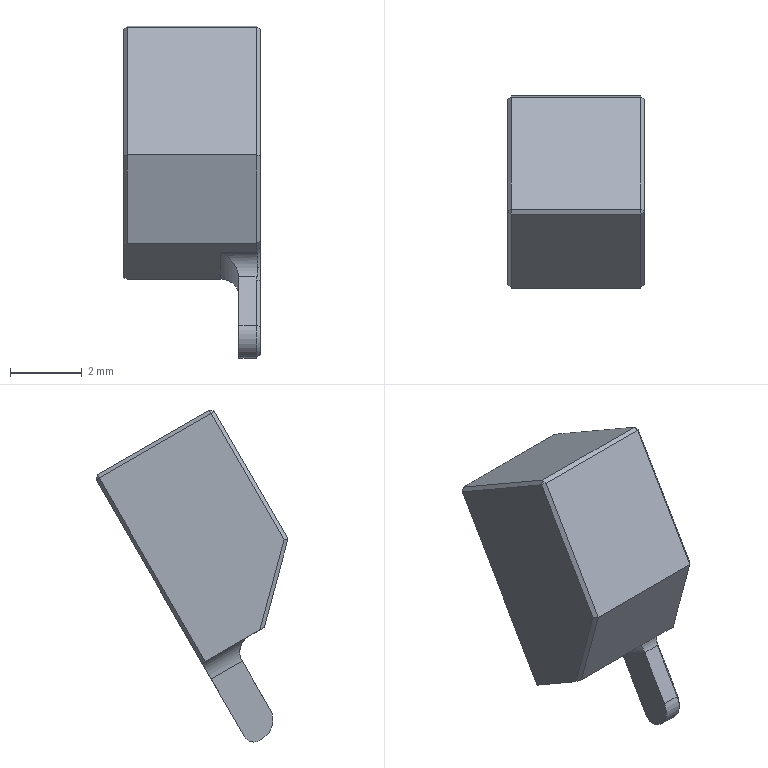Part | STEP file | 04-03 bending press head | 1 solid | 37 faces | box 3.8 x 5.341 x 9.237 mm | volume 81.885 mm3 | plane 28 | cylinder 7 | cone 2 | commonest cylinder face diameters 0.6 x2 1 x2 1.8 x2 1.2 x1
STEP:
#1=CARTESIAN_POINT('',(-4.131,-30.175,-1.884));
#2=VERTEX_POINT('',#1);
#3=CARTESIAN_POINT('',(-4.145,-30.425,-1.443));
#4=VERTEX_POINT('',#3);
#5=CARTESIAN_POINT('',(-4.131,-30.175,-1.884));
#6=CARTESIAN_POINT('',(-4.13,-30.173,-1.796));
#7=CARTESIAN_POINT('',(-4.13,-30.196,-1.707));
#8=CARTESIAN_POINT('',(-4.132,-30.284,-1.552));
#9=CARTESIAN_POINT('',(-4.134,-30.348,-1.487));
#10=CARTESIAN_POINT('',(-4.145,-30.425,-1.443));
#11=B_SPLINE_CURVE_WITH_KNOTS('',3,(#5,#6,#7,#8,#9,#10),.UNSPECIFIED.,.F.,.F.,(4,2,4),(0.0002526,0.0005174,0.0007821),.UNSPECIFIED.);
#12=EDGE_CURVE('',#2,#4,#11,.T.);
#13=ORIENTED_EDGE('',*,*,#12,.F.);
#14=CARTESIAN_POINT('',(-4.055,-30.07,-1.856));
#15=VERTEX_POINT('',#14);
#16=CARTESIAN_POINT('',(-3.632,-29.493,-1.702));
#17=DIRECTION('',(0.5774,0.7887,0.2113));
#18=VECTOR('',#17,1000.);
#19=LINE('',#16,#18);
#20=EDGE_CURVE('',#2,#15,#19,.T.);
#21=ORIENTED_EDGE('',*,*,#20,.T.);
#22=CARTESIAN_POINT('',(-4.055,-30.406,-1.338));
#23=VERTEX_POINT('',#22);
#24=CARTESIAN_POINT('',(-4.055,-30.406,-1.338));
#25=CARTESIAN_POINT('',(-4.055,-30.187,-1.465));
#26=CARTESIAN_POINT('',(-4.055,-30.07,-1.644));
#27=CARTESIAN_POINT('',(-4.055,-30.07,-1.856));
#28=(BOUNDED_CURVE()B_SPLINE_CURVE(3,(#24,#25,#26,#27),.UNSPECIFIED.,.F.,.F.)B_SPLINE_CURVE_WITH_KNOTS((4,4),(5.76,6.437),.UNSPECIFIED.)CURVE()GEOMETRIC_REPRESENTATION_ITEM()RATIONAL_B_SPLINE_CURVE((1.,0.9622,0.9622,1.))REPRESENTATION_ITEM(''));
#29=EDGE_CURVE('',#23,#15,#28,.T.);
#30=ORIENTED_EDGE('',*,*,#29,.F.);
#31=CARTESIAN_POINT('',(-4.155,-30.543,-1.375));
#32=VERTEX_POINT('',#31);
#33=CARTESIAN_POINT('',(-3.842,-30.117,-1.26));
#34=DIRECTION('',(0.5774,0.7887,0.2113));
#35=VECTOR('',#34,1000.);
#36=LINE('',#33,#35);
#37=EDGE_CURVE('',#32,#23,#36,.T.);
#38=ORIENTED_EDGE('',*,*,#37,.F.);
#39=CARTESIAN_POINT('',(-4.145,-30.425,-1.443));
#40=CARTESIAN_POINT('',(-4.152,-30.465,-1.42));
#41=CARTESIAN_POINT('',(-4.155,-30.505,-1.397));
#42=CARTESIAN_POINT('',(-4.155,-30.543,-1.375));
#43=(BOUNDED_CURVE()B_SPLINE_CURVE(3,(#39,#40,#41,#42),.UNSPECIFIED.,.F.,.F.)B_SPLINE_CURVE_WITH_KNOTS((4,4),(2.498,2.618),.UNSPECIFIED.)CURVE()GEOMETRIC_REPRESENTATION_ITEM()RATIONAL_B_SPLINE_CURVE((1.,0.9988,0.9988,1.))REPRESENTATION_ITEM(''));
#44=EDGE_CURVE('',#4,#32,#43,.T.);
#45=ORIENTED_EDGE('',*,*,#44,.F.);
#46=EDGE_LOOP('',(#13,#21,#30,#38,#45));
#47=FACE_OUTER_BOUND('',#46,.T.);
#48=CARTESIAN_POINT('',(-2.906,-30.025,-1.702));
#49=DIRECTION('',(0.5774,0.7887,0.2113));
#50=DIRECTION('',(-0.8069,0.5907,0.));
#51=AXIS2_PLACEMENT_3D('',#48,#49,#50);
#52=CYLINDRICAL_SURFACE('',#51,0.9);
#53=ADVANCED_FACE('',(#47),#52,.F.);
#54=CARTESIAN_POINT('',(-4.655,-30.714,-4.344));
#55=VERTEX_POINT('',#54);
#56=CARTESIAN_POINT('',(-4.655,-30.564,-4.384));
#57=VERTEX_POINT('',#56);
#58=CARTESIAN_POINT('',(-4.655,-30.564,-4.084));
#59=DIRECTION('',(1.,0.,0.));
#60=DIRECTION('',(0.,0.,-1.));
#61=AXIS2_PLACEMENT_3D('',#58,#59,#60);
#62=CIRCLE('',#61,0.3);
#63=EDGE_CURVE('',#55,#57,#62,.T.);
#64=ORIENTED_EDGE('',*,*,#63,.T.);
#65=CARTESIAN_POINT('',(-4.155,-30.564,-4.384));
#66=VERTEX_POINT('',#65);
#67=CARTESIAN_POINT('',(-4.655,-30.564,-4.384));
#68=DIRECTION('',(1.,0.,0.));
#69=VECTOR('',#68,1000.);
#70=LINE('',#67,#69);
#71=EDGE_CURVE('',#57,#66,#70,.T.);
#72=ORIENTED_EDGE('',*,*,#71,.T.);
#73=CARTESIAN_POINT('',(-4.155,-30.714,-4.344));
#74=VERTEX_POINT('',#73);
#75=CARTESIAN_POINT('',(-4.155,-30.564,-4.084));
#76=DIRECTION('',(-1.,0.,0.));
#77=DIRECTION('',(0.,0.,1.));
#78=AXIS2_PLACEMENT_3D('',#75,#76,#77);
#79=CIRCLE('',#78,0.3);
#80=EDGE_CURVE('',#66,#74,#79,.T.);
#81=ORIENTED_EDGE('',*,*,#80,.T.);
#82=CARTESIAN_POINT('',(-4.655,-30.714,-4.344));
#83=DIRECTION('',(1.,0.,0.));
#84=VECTOR('',#83,1000.);
#85=LINE('',#82,#84);
#86=EDGE_CURVE('',#55,#74,#85,.T.);
#87=ORIENTED_EDGE('',*,*,#86,.F.);
#88=EDGE_LOOP('',(#64,#72,#81,#87));
#89=FACE_OUTER_BOUND('',#88,.T.);
#90=CARTESIAN_POINT('',(-4.655,-30.564,-4.084));
#91=DIRECTION('',(1.,0.,0.));
#92=DIRECTION('',(0.,0.,-1.));
#93=AXIS2_PLACEMENT_3D('',#90,#91,#92);
#94=CYLINDRICAL_SURFACE('',#93,0.3);
#95=ADVANCED_FACE('',(#89),#94,.T.);
#96=CARTESIAN_POINT('',(-4.155,-29.33,4.853));
#97=VERTEX_POINT('',#96);
#98=CARTESIAN_POINT('',(-4.155,-26.212,3.053));
#99=VERTEX_POINT('',#98);
#100=CARTESIAN_POINT('',(-4.155,-26.126,3.003));
#101=DIRECTION('',(0.,0.866,-0.5));
#102=VECTOR('',#101,1000.);
#103=LINE('',#100,#102);
#104=EDGE_CURVE('',#97,#99,#103,.T.);
#105=ORIENTED_EDGE('',*,*,#104,.T.);
#106=CARTESIAN_POINT('',(-7.755,-26.212,3.053));
#107=VERTEX_POINT('',#106);
#108=CARTESIAN_POINT('',(-7.855,-26.212,3.053));
#109=DIRECTION('',(-1.,0.,0.));
#110=VECTOR('',#109,1000.);
#111=LINE('',#108,#110);
#112=EDGE_CURVE('',#99,#107,#111,.T.);
#113=ORIENTED_EDGE('',*,*,#112,.T.);
#114=CARTESIAN_POINT('',(-7.755,-29.33,4.853));
#115=VERTEX_POINT('',#114);
#116=CARTESIAN_POINT('',(-7.755,-29.417,4.903));
#117=DIRECTION('',(0.,-0.866,0.5));
#118=VECTOR('',#117,1000.);
#119=LINE('',#116,#118);
#120=EDGE_CURVE('',#107,#115,#119,.T.);
#121=ORIENTED_EDGE('',*,*,#120,.T.);
#122=CARTESIAN_POINT('',(-7.855,-29.33,4.853));
#123=DIRECTION('',(1.,0.,0.));
#124=VECTOR('',#123,1000.);
#125=LINE('',#122,#124);
#126=EDGE_CURVE('',#115,#97,#125,.T.);
#127=ORIENTED_EDGE('',*,*,#126,.T.);
#128=EDGE_LOOP('',(#105,#113,#121,#127));
#129=FACE_OUTER_BOUND('',#128,.T.);
#130=CARTESIAN_POINT('',(-7.855,-26.126,3.003));
#131=DIRECTION('',(0.,0.5,0.866));
#132=DIRECTION('',(0.,-0.866,0.5));
#133=AXIS2_PLACEMENT_3D('',#130,#131,#132);
#134=PLANE('',#133);
#135=ADVANCED_FACE('',(#129),#134,.T.);
#136=CARTESIAN_POINT('',(-4.155,-26.176,2.917));
#137=VERTEX_POINT('',#136);
#138=CARTESIAN_POINT('',(-4.155,-29.076,-2.106));
#139=VERTEX_POINT('',#138);
#140=CARTESIAN_POINT('',(-4.155,-29.126,-2.193));
#141=DIRECTION('',(0.,-0.5,-0.866));
#142=VECTOR('',#141,1000.);
#143=LINE('',#140,#142);
#144=EDGE_CURVE('',#137,#139,#143,.T.);
#145=ORIENTED_EDGE('',*,*,#144,.T.);
#146=CARTESIAN_POINT('',(-4.155,-30.304,-4.234));
#147=VERTEX_POINT('',#146);
#148=CARTESIAN_POINT('',(-4.155,-30.304,-4.234));
#149=DIRECTION('',(0.,-0.5,-0.866));
#150=VECTOR('',#149,1000.);
#151=LINE('',#148,#150);
#152=EDGE_CURVE('',#139,#147,#151,.T.);
#153=ORIENTED_EDGE('',*,*,#152,.T.);
#154=CARTESIAN_POINT('',(-4.655,-30.304,-4.234));
#155=VERTEX_POINT('',#154);
#156=CARTESIAN_POINT('',(-4.655,-30.304,-4.234));
#157=DIRECTION('',(1.,0.,0.));
#158=VECTOR('',#157,1000.);
#159=LINE('',#156,#158);
#160=EDGE_CURVE('',#155,#147,#159,.T.);
#161=ORIENTED_EDGE('',*,*,#160,.F.);
#162=CARTESIAN_POINT('',(-4.655,-29.376,-2.626));
#163=VERTEX_POINT('',#162);
#164=CARTESIAN_POINT('',(-4.655,-29.076,-2.106));
#165=DIRECTION('',(0.,0.5,0.866));
#166=VECTOR('',#165,1000.);
#167=LINE('',#164,#166);
#168=EDGE_CURVE('',#155,#163,#167,.T.);
#169=ORIENTED_EDGE('',*,*,#168,.T.);
#170=CARTESIAN_POINT('',(-5.155,-29.126,-2.193));
#171=VERTEX_POINT('',#170);
#172=CARTESIAN_POINT('',(-5.155,-29.376,-2.626));
#173=DIRECTION('',(0.,-0.866,0.5));
#174=DIRECTION('',(0.,0.5,0.866));
#175=AXIS2_PLACEMENT_3D('',#172,#173,#174);
#176=CIRCLE('',#175,0.5);
#177=EDGE_CURVE('',#163,#171,#176,.T.);
#178=ORIENTED_EDGE('',*,*,#177,.T.);
#179=CARTESIAN_POINT('',(-7.755,-29.126,-2.193));
#180=VERTEX_POINT('',#179);
#181=CARTESIAN_POINT('',(-4.055,-29.126,-2.193));
#182=DIRECTION('',(-1.,0.,0.));
#183=VECTOR('',#182,1000.);
#184=LINE('',#181,#183);
#185=EDGE_CURVE('',#171,#180,#184,.T.);
#186=ORIENTED_EDGE('',*,*,#185,.T.);
#187=CARTESIAN_POINT('',(-7.755,-26.176,2.917));
#188=VERTEX_POINT('',#187);
#189=CARTESIAN_POINT('',(-7.755,-26.126,3.003));
#190=DIRECTION('',(0.,0.5,0.866));
#191=VECTOR('',#190,1000.);
#192=LINE('',#189,#191);
#193=EDGE_CURVE('',#180,#188,#192,.T.);
#194=ORIENTED_EDGE('',*,*,#193,.T.);
#195=CARTESIAN_POINT('',(-7.855,-26.176,2.917));
#196=DIRECTION('',(1.,0.,0.));
#197=VECTOR('',#196,1000.);
#198=LINE('',#195,#197);
#199=EDGE_CURVE('',#188,#137,#198,.T.);
#200=ORIENTED_EDGE('',*,*,#199,.T.);
#201=EDGE_LOOP('',(#145,#153,#161,#169,#178,#186,#194,#200));
#202=FACE_OUTER_BOUND('',#201,.T.);
#203=CARTESIAN_POINT('',(-7.855,-30.454,-4.494));
#204=DIRECTION('',(0.,0.866,-0.5));
#205=DIRECTION('',(0.,0.5,0.866));
#206=AXIS2_PLACEMENT_3D('',#203,#204,#205);
#207=PLANE('',#206);
#208=ADVANCED_FACE('',(#202),#207,.T.);
#209=CARTESIAN_POINT('',(-4.155,-29.467,4.817));
#210=VERTEX_POINT('',#209);
#211=CARTESIAN_POINT('',(-7.755,-29.467,4.817));
#212=VERTEX_POINT('',#211);
#213=CARTESIAN_POINT('',(-7.855,-29.467,4.817));
#214=DIRECTION('',(-1.,0.,0.));
#215=VECTOR('',#214,1000.);
#216=LINE('',#213,#215);
#217=EDGE_CURVE('',#210,#212,#216,.T.);
#218=ORIENTED_EDGE('',*,*,#217,.T.);
#219=CARTESIAN_POINT('',(-7.755,-31.517,1.266));
#220=VERTEX_POINT('',#219);
#221=CARTESIAN_POINT('',(-7.755,-31.517,1.266));
#222=DIRECTION('',(0.,-0.5,-0.866));
#223=VECTOR('',#222,1000.);
#224=LINE('',#221,#223);
#225=EDGE_CURVE('',#212,#220,#224,.T.);
#226=ORIENTED_EDGE('',*,*,#225,.T.);
#227=CARTESIAN_POINT('',(-4.155,-31.517,1.266));
#228=VERTEX_POINT('',#227);
#229=CARTESIAN_POINT('',(-7.255,-31.517,1.266));
#230=DIRECTION('',(-1.,0.,0.));
#231=VECTOR('',#230,1000.);
#232=LINE('',#229,#231);
#233=EDGE_CURVE('',#228,#220,#232,.T.);
#234=ORIENTED_EDGE('',*,*,#233,.F.);
#235=CARTESIAN_POINT('',(-4.155,-29.417,4.903));
#236=DIRECTION('',(0.,0.5,0.866));
#237=VECTOR('',#236,1000.);
#238=LINE('',#235,#237);
#239=EDGE_CURVE('',#228,#210,#238,.T.);
#240=ORIENTED_EDGE('',*,*,#239,.T.);
#241=EDGE_LOOP('',(#218,#226,#234,#240));
#242=FACE_OUTER_BOUND('',#241,.T.);
#243=CARTESIAN_POINT('',(-7.855,-29.417,4.903));
#244=DIRECTION('',(0.,-0.866,0.5));
#245=DIRECTION('',(0.,-0.5,-0.866));
#246=AXIS2_PLACEMENT_3D('',#243,#244,#245);
#247=PLANE('',#246);
#248=ADVANCED_FACE('',(#242),#247,.T.);
#249=CARTESIAN_POINT('',(-7.855,-26.262,2.967));
#250=VERTEX_POINT('',#249);
#251=CARTESIAN_POINT('',(-7.855,-29.212,-2.143));
#252=VERTEX_POINT('',#251);
#253=CARTESIAN_POINT('',(-7.855,-30.391,-4.184));
#254=DIRECTION('',(0.,-0.5,-0.866));
#255=VECTOR('',#254,1000.);
#256=LINE('',#253,#255);
#257=EDGE_CURVE('',#250,#252,#256,.T.);
#258=ORIENTED_EDGE('',*,*,#257,.T.);
#259=CARTESIAN_POINT('',(-7.855,-30.735,-1.264));
#260=VERTEX_POINT('',#259);
#261=CARTESIAN_POINT('',(-7.855,-32.417,-0.2929));
#262=DIRECTION('',(0.,-0.866,0.5));
#263=VECTOR('',#262,1000.);
#264=LINE('',#261,#263);
#265=EDGE_CURVE('',#252,#260,#264,.T.);
#266=ORIENTED_EDGE('',*,*,#265,.T.);
#267=CARTESIAN_POINT('',(-7.855,-31.409,1.252));
#268=VERTEX_POINT('',#267);
#269=CARTESIAN_POINT('',(-7.855,-32.189,4.16));
#270=DIRECTION('',(0.,-0.2588,0.9659));
#271=VECTOR('',#270,1000.);
#272=LINE('',#269,#271);
#273=EDGE_CURVE('',#260,#268,#272,.T.);
#274=ORIENTED_EDGE('',*,*,#273,.T.);
#275=CARTESIAN_POINT('',(-7.855,-29.38,4.767));
#276=VERTEX_POINT('',#275);
#277=CARTESIAN_POINT('',(-7.855,-29.33,4.853));
#278=DIRECTION('',(0.,0.5,0.866));
#279=VECTOR('',#278,1000.);
#280=LINE('',#277,#279);
#281=EDGE_CURVE('',#268,#276,#280,.T.);
#282=ORIENTED_EDGE('',*,*,#281,.T.);
#283=CARTESIAN_POINT('',(-7.855,-26.176,2.917));
#284=DIRECTION('',(0.,0.866,-0.5));
#285=VECTOR('',#284,1000.);
#286=LINE('',#283,#285);
#287=EDGE_CURVE('',#276,#250,#286,.T.);
#288=ORIENTED_EDGE('',*,*,#287,.T.);
#289=EDGE_LOOP('',(#258,#266,#274,#282,#288));
#290=FACE_OUTER_BOUND('',#289,.T.);
#291=CARTESIAN_POINT('',(-7.855,-29.417,4.903));
#292=DIRECTION('',(1.,0.,0.));
#293=DIRECTION('',(0.,0.,-1.));
#294=AXIS2_PLACEMENT_3D('',#291,#292,#293);
#295=PLANE('',#294);
#296=ADVANCED_FACE('',(#290),#295,.F.);
#297=CARTESIAN_POINT('',(-7.755,-30.858,-1.193));
#298=VERTEX_POINT('',#297);
#299=CARTESIAN_POINT('',(-7.755,-31.517,1.266));
#300=DIRECTION('',(0.,0.2588,-0.9659));
#301=VECTOR('',#300,1000.);
#302=LINE('',#299,#301);
#303=EDGE_CURVE('',#220,#298,#302,.T.);
#304=ORIENTED_EDGE('',*,*,#303,.T.);
#305=CARTESIAN_POINT('',(-4.155,-30.858,-1.193));
#306=VERTEX_POINT('',#305);
#307=CARTESIAN_POINT('',(-4.055,-30.858,-1.193));
#308=DIRECTION('',(-1.,0.,0.));
#309=VECTOR('',#308,1000.);
#310=LINE('',#307,#309);
#311=EDGE_CURVE('',#306,#298,#310,.T.);
#312=ORIENTED_EDGE('',*,*,#311,.F.);
#313=CARTESIAN_POINT('',(-4.155,-31.517,1.266));
#314=DIRECTION('',(0.,-0.2588,0.9659));
#315=VECTOR('',#314,1000.);
#316=LINE('',#313,#315);
#317=EDGE_CURVE('',#306,#228,#316,.T.);
#318=ORIENTED_EDGE('',*,*,#317,.T.);
#319=ORIENTED_EDGE('',*,*,#233,.T.);
#320=EDGE_LOOP('',(#304,#312,#318,#319));
#321=FACE_OUTER_BOUND('',#320,.T.);
#322=CARTESIAN_POINT('',(-7.255,-31.517,1.266));
#323=DIRECTION('',(0.,0.9659,0.2588));
#324=DIRECTION('',(0.,-0.2588,0.9659));
#325=AXIS2_PLACEMENT_3D('',#322,#323,#324);
#326=PLANE('',#325);
#327=ADVANCED_FACE('',(#321),#326,.F.);
#328=ORIENTED_EDGE('',*,*,#185,.F.);
#329=CARTESIAN_POINT('',(-5.155,-30.425,-1.443));
#330=VERTEX_POINT('',#329);
#331=CARTESIAN_POINT('',(-5.155,-29.992,-1.693));
#332=DIRECTION('',(0.,-0.866,0.5));
#333=VECTOR('',#332,1000.);
#334=LINE('',#331,#333);
#335=EDGE_CURVE('',#171,#330,#334,.T.);
#336=ORIENTED_EDGE('',*,*,#335,.T.);
#337=CARTESIAN_POINT('',(-4.055,-30.425,-1.443));
#338=DIRECTION('',(1.,0.,0.));
#339=VECTOR('',#338,1000.);
#340=LINE('',#337,#339);
#341=EDGE_CURVE('',#330,#4,#340,.T.);
#342=ORIENTED_EDGE('',*,*,#341,.T.);
#343=ORIENTED_EDGE('',*,*,#44,.T.);
#344=CARTESIAN_POINT('',(-4.155,-29.126,-2.193));
#345=DIRECTION('',(0.,-0.866,0.5));
#346=VECTOR('',#345,1000.);
#347=LINE('',#344,#346);
#348=EDGE_CURVE('',#32,#306,#347,.T.);
#349=ORIENTED_EDGE('',*,*,#348,.T.);
#350=ORIENTED_EDGE('',*,*,#311,.T.);
#351=CARTESIAN_POINT('',(-6.906,-31.897,-0.5929));
#352=DIRECTION('',(-0.5774,0.7071,-0.4082));
#353=VECTOR('',#352,1000.);
#354=LINE('',#351,#353);
#355=EDGE_CURVE('',#298,#260,#354,.T.);
#356=ORIENTED_EDGE('',*,*,#355,.T.);
#357=ORIENTED_EDGE('',*,*,#265,.F.);
#358=CARTESIAN_POINT('',(-7.755,-29.126,-2.193));
#359=DIRECTION('',(0.7071,0.6124,-0.3536));
#360=VECTOR('',#359,1000.);
#361=LINE('',#358,#360);
#362=EDGE_CURVE('',#252,#180,#361,.T.);
#363=ORIENTED_EDGE('',*,*,#362,.T.);
#364=EDGE_LOOP('',(#328,#336,#342,#343,#349,#350,#356,#357,#363));
#365=FACE_OUTER_BOUND('',#364,.T.);
#366=CARTESIAN_POINT('',(-4.055,-29.126,-2.193));
#367=DIRECTION('',(0.,0.5,0.866));
#368=DIRECTION('',(0.,-0.866,0.5));
#369=AXIS2_PLACEMENT_3D('',#366,#367,#368);
#370=PLANE('',#369);
#371=ADVANCED_FACE('',(#365),#370,.F.);
#372=CARTESIAN_POINT('',(-4.055,-30.772,-1.127));
#373=VERTEX_POINT('',#372);
#374=CARTESIAN_POINT('',(-4.055,-29.076,-2.106));
#375=DIRECTION('',(0.,0.866,-0.5));
#376=VECTOR('',#375,1000.);
#377=LINE('',#374,#376);
#378=EDGE_CURVE('',#373,#23,#377,.T.);
#379=ORIENTED_EDGE('',*,*,#378,.T.);
#380=ORIENTED_EDGE('',*,*,#29,.T.);
#381=CARTESIAN_POINT('',(-4.055,-30.173,-2.207));
#382=VERTEX_POINT('',#381);
#383=CARTESIAN_POINT('',(-4.055,-30.07,-1.856));
#384=CARTESIAN_POINT('',(-4.055,-30.07,-1.971));
#385=CARTESIAN_POINT('',(-4.055,-30.105,-2.089));
#386=CARTESIAN_POINT('',(-4.055,-30.173,-2.207));
#387=(BOUNDED_CURVE()B_SPLINE_CURVE(3,(#383,#384,#385,#386),.UNSPECIFIED.,.F.,.F.)B_SPLINE_CURVE_WITH_KNOTS((4,4),(0.1535,0.5236),.UNSPECIFIED.)CURVE()GEOMETRIC_REPRESENTATION_ITEM()RATIONAL_B_SPLINE_CURVE((1.,0.9886,0.9886,1.))REPRESENTATION_ITEM(''));
#388=EDGE_CURVE('',#15,#382,#387,.T.);
#389=ORIENTED_EDGE('',*,*,#388,.T.);
#390=CARTESIAN_POINT('',(-4.055,-30.934,-3.524));
#391=VERTEX_POINT('',#390);
#392=CARTESIAN_POINT('',(-4.055,-30.934,-3.524));
#393=DIRECTION('',(0.,-0.5,-0.866));
#394=VECTOR('',#393,1000.);
#395=LINE('',#392,#394);
#396=EDGE_CURVE('',#382,#391,#395,.T.);
#397=ORIENTED_EDGE('',*,*,#396,.T.);
#398=CARTESIAN_POINT('',(-4.055,-30.751,-4.207));
#399=VERTEX_POINT('',#398);
#400=CARTESIAN_POINT('',(-4.055,-30.501,-3.774));
#401=DIRECTION('',(1.,0.,0.));
#402=DIRECTION('',(0.,0.,1.));
#403=AXIS2_PLACEMENT_3D('',#400,#401,#402);
#404=CIRCLE('',#403,0.5);
#405=EDGE_CURVE('',#391,#399,#404,.T.);
#406=ORIENTED_EDGE('',*,*,#405,.T.);
#407=CARTESIAN_POINT('',(-4.055,-30.664,-4.257));
#408=VERTEX_POINT('',#407);
#409=CARTESIAN_POINT('',(-4.055,-30.664,-4.257));
#410=DIRECTION('',(0.,0.866,-0.5));
#411=VECTOR('',#410,1000.);
#412=LINE('',#409,#411);
#413=EDGE_CURVE('',#399,#408,#412,.T.);
#414=ORIENTED_EDGE('',*,*,#413,.T.);
#415=CARTESIAN_POINT('',(-4.055,-30.391,-4.184));
#416=VERTEX_POINT('',#415);
#417=CARTESIAN_POINT('',(-4.055,-30.564,-4.084));
#418=DIRECTION('',(1.,0.,0.));
#419=DIRECTION('',(0.,0.,1.));
#420=AXIS2_PLACEMENT_3D('',#417,#418,#419);
#421=CIRCLE('',#420,0.2);
#422=EDGE_CURVE('',#408,#416,#421,.T.);
#423=ORIENTED_EDGE('',*,*,#422,.T.);
#424=CARTESIAN_POINT('',(-4.055,-29.162,-2.056));
#425=VERTEX_POINT('',#424);
#426=CARTESIAN_POINT('',(-4.055,-29.162,-2.056));
#427=DIRECTION('',(0.,0.5,0.866));
#428=VECTOR('',#427,1000.);
#429=LINE('',#426,#428);
#430=EDGE_CURVE('',#416,#425,#429,.T.);
#431=ORIENTED_EDGE('',*,*,#430,.T.);
#432=CARTESIAN_POINT('',(-4.055,-26.262,2.967));
#433=VERTEX_POINT('',#432);
#434=CARTESIAN_POINT('',(-4.055,-26.212,3.053));
#435=DIRECTION('',(0.,0.5,0.866));
#436=VECTOR('',#435,1000.);
#437=LINE('',#434,#436);
#438=EDGE_CURVE('',#425,#433,#437,.T.);
#439=ORIENTED_EDGE('',*,*,#438,.T.);
#440=CARTESIAN_POINT('',(-4.055,-29.38,4.767));
#441=VERTEX_POINT('',#440);
#442=CARTESIAN_POINT('',(-4.055,-29.467,4.817));
#443=DIRECTION('',(0.,-0.866,0.5));
#444=VECTOR('',#443,1000.);
#445=LINE('',#442,#444);
#446=EDGE_CURVE('',#433,#441,#445,.T.);
#447=ORIENTED_EDGE('',*,*,#446,.T.);
#448=CARTESIAN_POINT('',(-4.055,-31.409,1.252));
#449=VERTEX_POINT('',#448);
#450=CARTESIAN_POINT('',(-4.055,-31.43,1.216));
#451=DIRECTION('',(0.,-0.5,-0.866));
#452=VECTOR('',#451,1000.);
#453=LINE('',#450,#452);
#454=EDGE_CURVE('',#441,#449,#453,.T.);
#455=ORIENTED_EDGE('',*,*,#454,.T.);
#456=CARTESIAN_POINT('',(-4.055,-31.493,1.565));
#457=DIRECTION('',(0.,0.2588,-0.9659));
#458=VECTOR('',#457,1000.);
#459=LINE('',#456,#458);
#460=EDGE_CURVE('',#449,#373,#459,.T.);
#461=ORIENTED_EDGE('',*,*,#460,.T.);
#462=EDGE_LOOP('',(#379,#380,#389,#397,#406,#414,#423,#431,#439,#447,#455,#461));
#463=FACE_OUTER_BOUND('',#462,.T.);
#464=CARTESIAN_POINT('',(-4.055,-26.126,3.003));
#465=DIRECTION('',(-1.,0.,0.));
#466=DIRECTION('',(0.,0.,1.));
#467=AXIS2_PLACEMENT_3D('',#464,#465,#466);
#468=PLANE('',#467);
#469=ADVANCED_FACE('',(#463),#468,.F.);
#470=CARTESIAN_POINT('',(-3.523,-30.316,-0.7767));
#471=DIRECTION('',(-0.6786,-0.5827,-0.4471));
#472=VECTOR('',#471,1000.);
#473=LINE('',#470,#472);
#474=EDGE_CURVE('',#373,#306,#473,.T.);
#475=ORIENTED_EDGE('',*,*,#474,.F.);
#476=ORIENTED_EDGE('',*,*,#460,.F.);
#477=CARTESIAN_POINT('',(-3.261,-30.558,1.14));
#478=DIRECTION('',(0.6786,0.7282,-0.09587));
#479=VECTOR('',#478,1000.);
#480=LINE('',#477,#479);
#481=EDGE_CURVE('',#228,#449,#480,.T.);
#482=ORIENTED_EDGE('',*,*,#481,.F.);
#483=ORIENTED_EDGE('',*,*,#317,.F.);
#484=EDGE_LOOP('',(#475,#476,#482,#483));
#485=FACE_OUTER_BOUND('',#484,.T.);
#486=CARTESIAN_POINT('',(-4.055,-31.493,1.565));
#487=DIRECTION('',(-0.7071,0.683,0.183));
#488=DIRECTION('',(-0.6947,-0.7193,0.));
#489=AXIS2_PLACEMENT_3D('',#486,#487,#488);
#490=PLANE('',#489);
#491=ADVANCED_FACE('',(#485),#490,.F.);
#492=ORIENTED_EDGE('',*,*,#481,.T.);
#493=ORIENTED_EDGE('',*,*,#454,.F.);
#494=CARTESIAN_POINT('',(-4.155,-29.467,4.817));
#495=DIRECTION('',(0.7071,0.6124,-0.3536));
#496=VECTOR('',#495,1000.);
#497=LINE('',#494,#496);
#498=EDGE_CURVE('',#210,#441,#497,.T.);
#499=ORIENTED_EDGE('',*,*,#498,.F.);
#500=ORIENTED_EDGE('',*,*,#239,.F.);
#501=EDGE_LOOP('',(#492,#493,#499,#500));
#502=FACE_OUTER_BOUND('',#501,.T.);
#503=CARTESIAN_POINT('',(-4.055,-29.33,4.853));
#504=DIRECTION('',(0.7071,-0.6124,0.3536));
#505=DIRECTION('',(0.6547,0.7559,0.));
#506=AXIS2_PLACEMENT_3D('',#503,#504,#505);
#507=PLANE('',#506);
#508=ADVANCED_FACE('',(#502),#507,.T.);
#509=ORIENTED_EDGE('',*,*,#348,.F.);
#510=ORIENTED_EDGE('',*,*,#37,.T.);
#511=ORIENTED_EDGE('',*,*,#378,.F.);
#512=ORIENTED_EDGE('',*,*,#474,.T.);
#513=EDGE_LOOP('',(#509,#510,#511,#512));
#514=FACE_OUTER_BOUND('',#513,.T.);
#515=CARTESIAN_POINT('',(-4.055,-29.076,-2.106));
#516=DIRECTION('',(-0.7071,0.3536,0.6124));
#517=DIRECTION('',(0.6547,0.,0.7559));
#518=AXIS2_PLACEMENT_3D('',#515,#516,#517);
#519=PLANE('',#518);
#520=ADVANCED_FACE('',(#514),#519,.F.);
#521=CARTESIAN_POINT('',(-4.155,-29.467,4.817));
#522=DIRECTION('',(0.,0.9659,0.2588));
#523=VECTOR('',#522,1000.);
#524=LINE('',#521,#523);
#525=EDGE_CURVE('',#210,#97,#524,.T.);
#526=ORIENTED_EDGE('',*,*,#525,.F.);
#527=ORIENTED_EDGE('',*,*,#498,.T.);
#528=CARTESIAN_POINT('',(-4.105,-29.355,4.81));
#529=DIRECTION('',(0.7071,-0.3536,-0.6124));
#530=VECTOR('',#529,1000.);
#531=LINE('',#528,#530);
#532=EDGE_CURVE('',#97,#441,#531,.T.);
#533=ORIENTED_EDGE('',*,*,#532,.F.);
#534=EDGE_LOOP('',(#526,#527,#533));
#535=FACE_OUTER_BOUND('',#534,.T.);
#536=CARTESIAN_POINT('',(-4.155,-29.467,4.817));
#537=DIRECTION('',(0.5774,-0.2113,0.7887));
#538=DIRECTION('',(0.8069,0.,-0.5907));
#539=AXIS2_PLACEMENT_3D('',#536,#537,#538);
#540=PLANE('',#539);
#541=ADVANCED_FACE('',(#535),#540,.T.);
#542=CARTESIAN_POINT('',(-4.055,-29.162,-2.056));
#543=DIRECTION('',(0.7071,-0.6124,0.3536));
#544=VECTOR('',#543,1000.);
#545=LINE('',#542,#544);
#546=EDGE_CURVE('',#139,#425,#545,.T.);
#547=ORIENTED_EDGE('',*,*,#546,.F.);
#548=ORIENTED_EDGE('',*,*,#144,.F.);
#549=CARTESIAN_POINT('',(-4.155,-26.176,2.917));
#550=DIRECTION('',(-0.7071,0.6124,-0.3536));
#551=VECTOR('',#550,1000.);
#552=LINE('',#549,#551);
#553=EDGE_CURVE('',#433,#137,#552,.T.);
#554=ORIENTED_EDGE('',*,*,#553,.F.);
#555=ORIENTED_EDGE('',*,*,#438,.F.);
#556=EDGE_LOOP('',(#547,#548,#554,#555));
#557=FACE_OUTER_BOUND('',#556,.T.);
#558=CARTESIAN_POINT('',(-4.055,-26.212,3.053));
#559=DIRECTION('',(0.7071,0.6124,-0.3536));
#560=DIRECTION('',(-0.6547,0.7559,0.));
#561=AXIS2_PLACEMENT_3D('',#558,#559,#560);
#562=PLANE('',#561);
#563=ADVANCED_FACE('',(#557),#562,.T.);
#564=ORIENTED_EDGE('',*,*,#532,.T.);
#565=ORIENTED_EDGE('',*,*,#446,.F.);
#566=CARTESIAN_POINT('',(-4.105,-26.237,3.01));
#567=DIRECTION('',(0.7071,-0.3536,-0.6124));
#568=VECTOR('',#567,1000.);
#569=LINE('',#566,#568);
#570=EDGE_CURVE('',#99,#433,#569,.T.);
#571=ORIENTED_EDGE('',*,*,#570,.F.);
#572=ORIENTED_EDGE('',*,*,#104,.F.);
#573=EDGE_LOOP('',(#564,#565,#571,#572));
#574=FACE_OUTER_BOUND('',#573,.T.);
#575=CARTESIAN_POINT('',(-4.055,-26.176,2.917));
#576=DIRECTION('',(0.7071,0.3536,0.6124));
#577=DIRECTION('',(0.6547,0.,-0.7559));
#578=AXIS2_PLACEMENT_3D('',#575,#576,#577);
#579=PLANE('',#578);
#580=ADVANCED_FACE('',(#574),#579,.T.);
#581=ORIENTED_EDGE('',*,*,#525,.T.);
#582=ORIENTED_EDGE('',*,*,#126,.F.);
#583=CARTESIAN_POINT('',(-7.755,-29.398,4.835));
#584=DIRECTION('',(0.,0.9659,0.2588));
#585=VECTOR('',#584,1000.);
#586=LINE('',#583,#585);
#587=EDGE_CURVE('',#212,#115,#586,.T.);
#588=ORIENTED_EDGE('',*,*,#587,.F.);
#589=ORIENTED_EDGE('',*,*,#217,.F.);
#590=EDGE_LOOP('',(#581,#582,#588,#589));
#591=FACE_OUTER_BOUND('',#590,.T.);
#592=CARTESIAN_POINT('',(-7.855,-29.33,4.853));
#593=DIRECTION('',(0.,0.2588,-0.9659));
#594=DIRECTION('',(0.,0.9659,0.2588));
#595=AXIS2_PLACEMENT_3D('',#592,#593,#594);
#596=PLANE('',#595);
#597=ADVANCED_FACE('',(#591),#596,.F.);
#598=ORIENTED_EDGE('',*,*,#570,.T.);
#599=ORIENTED_EDGE('',*,*,#553,.T.);
#600=CARTESIAN_POINT('',(-4.155,-26.176,2.917));
#601=DIRECTION('',(0.,0.2588,-0.9659));
#602=VECTOR('',#601,1000.);
#603=LINE('',#600,#602);
#604=EDGE_CURVE('',#99,#137,#603,.T.);
#605=ORIENTED_EDGE('',*,*,#604,.F.);
#606=EDGE_LOOP('',(#598,#599,#605));
#607=FACE_OUTER_BOUND('',#606,.T.);
#608=CARTESIAN_POINT('',(-4.155,-26.176,2.917));
#609=DIRECTION('',(0.5774,0.7887,0.2113));
#610=DIRECTION('',(-0.8069,0.5907,0.));
#611=AXIS2_PLACEMENT_3D('',#608,#609,#610);
#612=PLANE('',#611);
#613=ADVANCED_FACE('',(#607),#612,.T.);
#614=CARTESIAN_POINT('',(-7.855,-29.38,4.767));
#615=DIRECTION('',(0.7071,0.3536,0.6124));
#616=VECTOR('',#615,1000.);
#617=LINE('',#614,#616);
#618=EDGE_CURVE('',#276,#115,#617,.T.);
#619=ORIENTED_EDGE('',*,*,#618,.F.);
#620=CARTESIAN_POINT('',(-7.855,-29.38,4.767));
#621=DIRECTION('',(-0.7071,0.6124,-0.3536));
#622=VECTOR('',#621,1000.);
#623=LINE('',#620,#622);
#624=EDGE_CURVE('',#212,#276,#623,.T.);
#625=ORIENTED_EDGE('',*,*,#624,.F.);
#626=ORIENTED_EDGE('',*,*,#587,.T.);
#627=EDGE_LOOP('',(#619,#625,#626));
#628=FACE_OUTER_BOUND('',#627,.T.);
#629=CARTESIAN_POINT('',(-7.855,-29.38,4.767));
#630=DIRECTION('',(-0.5774,-0.2113,0.7887));
#631=DIRECTION('',(0.8069,0.,0.5907));
#632=AXIS2_PLACEMENT_3D('',#629,#630,#631);
#633=PLANE('',#632);
#634=ADVANCED_FACE('',(#628),#633,.T.);
#635=ORIENTED_EDGE('',*,*,#624,.T.);
#636=ORIENTED_EDGE('',*,*,#281,.F.);
#637=CARTESIAN_POINT('',(-8.556,-30.657,1.153));
#638=DIRECTION('',(-0.6786,0.7282,-0.09587));
#639=VECTOR('',#638,1000.);
#640=LINE('',#637,#639);
#641=EDGE_CURVE('',#220,#268,#640,.T.);
#642=ORIENTED_EDGE('',*,*,#641,.F.);
#643=ORIENTED_EDGE('',*,*,#225,.F.);
#644=EDGE_LOOP('',(#635,#636,#642,#643));
#645=FACE_OUTER_BOUND('',#644,.T.);
#646=CARTESIAN_POINT('',(-7.755,-29.417,4.903));
#647=DIRECTION('',(-0.7071,-0.6124,0.3536));
#648=DIRECTION('',(0.6547,-0.7559,0.));
#649=AXIS2_PLACEMENT_3D('',#646,#647,#648);
#650=PLANE('',#649);
#651=ADVANCED_FACE('',(#645),#650,.T.);
#652=ORIENTED_EDGE('',*,*,#604,.T.);
#653=ORIENTED_EDGE('',*,*,#199,.F.);
#654=CARTESIAN_POINT('',(-7.755,-26.176,2.917));
#655=DIRECTION('',(0.,0.2588,-0.9659));
#656=VECTOR('',#655,1000.);
#657=LINE('',#654,#656);
#658=EDGE_CURVE('',#107,#188,#657,.T.);
#659=ORIENTED_EDGE('',*,*,#658,.F.);
#660=ORIENTED_EDGE('',*,*,#112,.F.);
#661=EDGE_LOOP('',(#652,#653,#659,#660));
#662=FACE_OUTER_BOUND('',#661,.T.);
#663=CARTESIAN_POINT('',(-7.855,-26.176,2.917));
#664=DIRECTION('',(0.,-0.9659,-0.2588));
#665=DIRECTION('',(0.,0.2588,-0.9659));
#666=AXIS2_PLACEMENT_3D('',#663,#664,#665);
#667=PLANE('',#666);
#668=ADVANCED_FACE('',(#662),#667,.F.);
#669=ORIENTED_EDGE('',*,*,#618,.T.);
#670=ORIENTED_EDGE('',*,*,#120,.F.);
#671=CARTESIAN_POINT('',(-7.805,-26.237,3.01));
#672=DIRECTION('',(0.7071,0.3536,0.6124));
#673=VECTOR('',#672,1000.);
#674=LINE('',#671,#673);
#675=EDGE_CURVE('',#250,#107,#674,.T.);
#676=ORIENTED_EDGE('',*,*,#675,.F.);
#677=ORIENTED_EDGE('',*,*,#287,.F.);
#678=EDGE_LOOP('',(#669,#670,#676,#677));
#679=FACE_OUTER_BOUND('',#678,.T.);
#680=CARTESIAN_POINT('',(-7.755,-26.126,3.003));
#681=DIRECTION('',(-0.7071,0.3536,0.6124));
#682=DIRECTION('',(0.6547,0.,0.7559));
#683=AXIS2_PLACEMENT_3D('',#680,#681,#682);
#684=PLANE('',#683);
#685=ADVANCED_FACE('',(#679),#684,.T.);
#686=ORIENTED_EDGE('',*,*,#355,.F.);
#687=ORIENTED_EDGE('',*,*,#303,.F.);
#688=ORIENTED_EDGE('',*,*,#641,.T.);
#689=ORIENTED_EDGE('',*,*,#273,.F.);
#690=EDGE_LOOP('',(#686,#687,#688,#689));
#691=FACE_OUTER_BOUND('',#690,.T.);
#692=CARTESIAN_POINT('',(-7.755,-31.517,1.266));
#693=DIRECTION('',(0.7071,0.683,0.183));
#694=DIRECTION('',(-0.6947,0.7193,0.));
#695=AXIS2_PLACEMENT_3D('',#692,#693,#694);
#696=PLANE('',#695);
#697=ADVANCED_FACE('',(#691),#696,.F.);
#698=ORIENTED_EDGE('',*,*,#675,.T.);
#699=ORIENTED_EDGE('',*,*,#658,.T.);
#700=CARTESIAN_POINT('',(-7.755,-26.176,2.917));
#701=DIRECTION('',(0.7071,0.6124,-0.3536));
#702=VECTOR('',#701,1000.);
#703=LINE('',#700,#702);
#704=EDGE_CURVE('',#250,#188,#703,.T.);
#705=ORIENTED_EDGE('',*,*,#704,.F.);
#706=EDGE_LOOP('',(#698,#699,#705));
#707=FACE_OUTER_BOUND('',#706,.T.);
#708=CARTESIAN_POINT('',(-7.755,-26.176,2.917));
#709=DIRECTION('',(-0.5774,0.7887,0.2113));
#710=DIRECTION('',(-0.8069,-0.5907,0.));
#711=AXIS2_PLACEMENT_3D('',#708,#709,#710);
#712=PLANE('',#711);
#713=ADVANCED_FACE('',(#707),#712,.T.);
#714=ORIENTED_EDGE('',*,*,#362,.F.);
#715=ORIENTED_EDGE('',*,*,#257,.F.);
#716=ORIENTED_EDGE('',*,*,#704,.T.);
#717=ORIENTED_EDGE('',*,*,#193,.F.);
#718=EDGE_LOOP('',(#714,#715,#716,#717));
#719=FACE_OUTER_BOUND('',#718,.T.);
#720=CARTESIAN_POINT('',(-7.755,-30.454,-4.494));
#721=DIRECTION('',(-0.7071,0.6124,-0.3536));
#722=DIRECTION('',(-0.6547,-0.7559,0.));
#723=AXIS2_PLACEMENT_3D('',#720,#721,#722);
#724=PLANE('',#723);
#725=ADVANCED_FACE('',(#719),#724,.T.);
#726=CARTESIAN_POINT('',(-4.655,-30.242,-2.126));
#727=VERTEX_POINT('',#726);
#728=CARTESIAN_POINT('',(-4.655,-31.02,-3.474));
#729=VERTEX_POINT('',#728);
#730=CARTESIAN_POINT('',(-4.655,-31.02,-3.474));
#731=DIRECTION('',(0.,-0.5,-0.866));
#732=VECTOR('',#731,1000.);
#733=LINE('',#730,#732);
#734=EDGE_CURVE('',#727,#729,#733,.T.);
#735=ORIENTED_EDGE('',*,*,#734,.F.);
#736=CARTESIAN_POINT('',(-4.655,-29.376,-2.626));
#737=DIRECTION('',(0.,0.866,-0.5));
#738=VECTOR('',#737,1000.);
#739=LINE('',#736,#738);
#740=EDGE_CURVE('',#727,#163,#739,.T.);
#741=ORIENTED_EDGE('',*,*,#740,.T.);
#742=ORIENTED_EDGE('',*,*,#168,.F.);
#743=CARTESIAN_POINT('',(-4.655,-30.564,-4.084));
#744=DIRECTION('',(1.,0.,0.));
#745=DIRECTION('',(0.,0.,-1.));
#746=AXIS2_PLACEMENT_3D('',#743,#744,#745);
#747=CIRCLE('',#746,0.3);
#748=EDGE_CURVE('',#57,#155,#747,.T.);
#749=ORIENTED_EDGE('',*,*,#748,.F.);
#750=ORIENTED_EDGE('',*,*,#63,.F.);
#751=CARTESIAN_POINT('',(-4.655,-30.801,-4.294));
#752=VERTEX_POINT('',#751);
#753=CARTESIAN_POINT('',(-4.655,-30.714,-4.344));
#754=DIRECTION('',(0.,0.866,-0.5));
#755=VECTOR('',#754,1000.);
#756=LINE('',#753,#755);
#757=EDGE_CURVE('',#752,#55,#756,.T.);
#758=ORIENTED_EDGE('',*,*,#757,.F.);
#759=CARTESIAN_POINT('',(-4.655,-30.501,-3.774));
#760=DIRECTION('',(1.,0.,0.));
#761=DIRECTION('',(0.,0.,-1.));
#762=AXIS2_PLACEMENT_3D('',#759,#760,#761);
#763=CIRCLE('',#762,0.6);
#764=EDGE_CURVE('',#729,#752,#763,.T.);
#765=ORIENTED_EDGE('',*,*,#764,.F.);
#766=EDGE_LOOP('',(#735,#741,#742,#749,#750,#758,#765));
#767=FACE_OUTER_BOUND('',#766,.T.);
#768=CARTESIAN_POINT('',(-4.655,-30.564,-4.084));
#769=DIRECTION('',(1.,0.,0.));
#770=DIRECTION('',(0.,0.,-1.));
#771=AXIS2_PLACEMENT_3D('',#768,#769,#770);
#772=PLANE('',#771);
#773=ADVANCED_FACE('',(#767),#772,.F.);
#774=CARTESIAN_POINT('',(-4.155,-31.02,-3.474));
#775=VERTEX_POINT('',#774);
#776=CARTESIAN_POINT('',(-4.155,-30.31,-2.244));
#777=VERTEX_POINT('',#776);
#778=CARTESIAN_POINT('',(-4.155,-29.942,-1.606));
#779=DIRECTION('',(0.,0.5,0.866));
#780=VECTOR('',#779,1000.);
#781=LINE('',#778,#780);
#782=EDGE_CURVE('',#775,#777,#781,.T.);
#783=ORIENTED_EDGE('',*,*,#782,.T.);
#784=CARTESIAN_POINT('',(-4.145,-30.242,-2.126));
#785=VERTEX_POINT('',#784);
#786=CARTESIAN_POINT('',(-4.155,-30.31,-2.244));
#787=CARTESIAN_POINT('',(-4.155,-30.288,-2.206));
#788=CARTESIAN_POINT('',(-4.152,-30.265,-2.166));
#789=CARTESIAN_POINT('',(-4.145,-30.242,-2.126));
#790=(BOUNDED_CURVE()B_SPLINE_CURVE(3,(#786,#787,#788,#789),.UNSPECIFIED.,.F.,.F.)B_SPLINE_CURVE_WITH_KNOTS((4,4),(3.665,3.785),.UNSPECIFIED.)CURVE()GEOMETRIC_REPRESENTATION_ITEM()RATIONAL_B_SPLINE_CURVE((1.,0.9988,0.9988,1.))REPRESENTATION_ITEM(''));
#791=EDGE_CURVE('',#777,#785,#790,.T.);
#792=ORIENTED_EDGE('',*,*,#791,.T.);
#793=CARTESIAN_POINT('',(-4.655,-30.242,-2.126));
#794=DIRECTION('',(-1.,0.,0.));
#795=VECTOR('',#794,1000.);
#796=LINE('',#793,#795);
#797=EDGE_CURVE('',#785,#727,#796,.T.);
#798=ORIENTED_EDGE('',*,*,#797,.T.);
#799=ORIENTED_EDGE('',*,*,#734,.T.);
#800=CARTESIAN_POINT('',(-4.655,-31.02,-3.474));
#801=DIRECTION('',(1.,0.,0.));
#802=VECTOR('',#801,1000.);
#803=LINE('',#800,#802);
#804=EDGE_CURVE('',#729,#775,#803,.T.);
#805=ORIENTED_EDGE('',*,*,#804,.T.);
#806=EDGE_LOOP('',(#783,#792,#798,#799,#805));
#807=FACE_OUTER_BOUND('',#806,.T.);
#808=CARTESIAN_POINT('',(-4.655,-31.02,-3.474));
#809=DIRECTION('',(0.,-0.866,0.5));
#810=DIRECTION('',(0.,-0.5,-0.866));
#811=AXIS2_PLACEMENT_3D('',#808,#809,#810);
#812=PLANE('',#811);
#813=ADVANCED_FACE('',(#807),#812,.T.);
#814=ORIENTED_EDGE('',*,*,#71,.F.);
#815=ORIENTED_EDGE('',*,*,#748,.T.);
#816=ORIENTED_EDGE('',*,*,#160,.T.);
#817=CARTESIAN_POINT('',(-4.155,-30.564,-4.084));
#818=DIRECTION('',(-1.,0.,0.));
#819=DIRECTION('',(0.,0.,1.));
#820=AXIS2_PLACEMENT_3D('',#817,#818,#819);
#821=CIRCLE('',#820,0.3);
#822=EDGE_CURVE('',#147,#66,#821,.T.);
#823=ORIENTED_EDGE('',*,*,#822,.T.);
#824=EDGE_LOOP('',(#814,#815,#816,#823));
#825=FACE_OUTER_BOUND('',#824,.T.);
#826=CARTESIAN_POINT('',(-4.655,-30.564,-4.084));
#827=DIRECTION('',(1.,0.,0.));
#828=DIRECTION('',(0.,0.,-1.));
#829=AXIS2_PLACEMENT_3D('',#826,#827,#828);
#830=CYLINDRICAL_SURFACE('',#829,0.3);
#831=ADVANCED_FACE('',(#825),#830,.T.);
#832=ORIENTED_EDGE('',*,*,#86,.T.);
#833=CARTESIAN_POINT('',(-4.155,-30.801,-4.294));
#834=VERTEX_POINT('',#833);
#835=CARTESIAN_POINT('',(-4.155,-30.801,-4.294));
#836=DIRECTION('',(0.,-0.866,0.5));
#837=VECTOR('',#836,1000.);
#838=LINE('',#835,#837);
#839=EDGE_CURVE('',#74,#834,#838,.T.);
#840=ORIENTED_EDGE('',*,*,#839,.T.);
#841=CARTESIAN_POINT('',(-4.655,-30.801,-4.294));
#842=DIRECTION('',(1.,0.,0.));
#843=VECTOR('',#842,1000.);
#844=LINE('',#841,#843);
#845=EDGE_CURVE('',#752,#834,#844,.T.);
#846=ORIENTED_EDGE('',*,*,#845,.F.);
#847=ORIENTED_EDGE('',*,*,#757,.T.);
#848=EDGE_LOOP('',(#832,#840,#846,#847));
#849=FACE_OUTER_BOUND('',#848,.T.);
#850=CARTESIAN_POINT('',(-4.655,-30.714,-4.344));
#851=DIRECTION('',(0.,-0.5,-0.866));
#852=DIRECTION('',(0.,0.866,-0.5));
#853=AXIS2_PLACEMENT_3D('',#850,#851,#852);
#854=PLANE('',#853);
#855=ADVANCED_FACE('',(#849),#854,.T.);
#856=ORIENTED_EDGE('',*,*,#845,.T.);
#857=CARTESIAN_POINT('',(-4.155,-30.501,-3.774));
#858=DIRECTION('',(-1.,0.,0.));
#859=DIRECTION('',(0.,0.,1.));
#860=AXIS2_PLACEMENT_3D('',#857,#858,#859);
#861=CIRCLE('',#860,0.6);
#862=EDGE_CURVE('',#834,#775,#861,.T.);
#863=ORIENTED_EDGE('',*,*,#862,.T.);
#864=ORIENTED_EDGE('',*,*,#804,.F.);
#865=ORIENTED_EDGE('',*,*,#764,.T.);
#866=EDGE_LOOP('',(#856,#863,#864,#865));
#867=FACE_OUTER_BOUND('',#866,.T.);
#868=CARTESIAN_POINT('',(-4.655,-30.501,-3.774));
#869=DIRECTION('',(1.,0.,0.));
#870=DIRECTION('',(0.,0.,-1.));
#871=AXIS2_PLACEMENT_3D('',#868,#869,#870);
#872=CYLINDRICAL_SURFACE('',#871,0.6);
#873=ADVANCED_FACE('',(#867),#872,.T.);
#874=ORIENTED_EDGE('',*,*,#546,.T.);
#875=ORIENTED_EDGE('',*,*,#430,.F.);
#876=CARTESIAN_POINT('',(-4.155,-30.304,-4.234));
#877=DIRECTION('',(0.7071,-0.6124,0.3536));
#878=VECTOR('',#877,1000.);
#879=LINE('',#876,#878);
#880=EDGE_CURVE('',#147,#416,#879,.T.);
#881=ORIENTED_EDGE('',*,*,#880,.F.);
#882=ORIENTED_EDGE('',*,*,#152,.F.);
#883=EDGE_LOOP('',(#874,#875,#881,#882));
#884=FACE_OUTER_BOUND('',#883,.T.);
#885=CARTESIAN_POINT('',(-4.055,-26.212,3.053));
#886=DIRECTION('',(0.7071,0.6124,-0.3536));
#887=DIRECTION('',(-0.6547,0.7559,0.));
#888=AXIS2_PLACEMENT_3D('',#885,#886,#887);
#889=PLANE('',#888);
#890=ADVANCED_FACE('',(#884),#889,.T.);
#891=ORIENTED_EDGE('',*,*,#880,.T.);
#892=ORIENTED_EDGE('',*,*,#422,.F.);
#893=CARTESIAN_POINT('',(-4.155,-30.714,-4.344));
#894=DIRECTION('',(0.7071,0.3536,0.6124));
#895=VECTOR('',#894,1000.);
#896=LINE('',#893,#895);
#897=EDGE_CURVE('',#74,#408,#896,.T.);
#898=ORIENTED_EDGE('',*,*,#897,.F.);
#899=ORIENTED_EDGE('',*,*,#80,.F.);
#900=ORIENTED_EDGE('',*,*,#822,.F.);
#901=EDGE_LOOP('',(#891,#892,#898,#899,#900));
#902=FACE_OUTER_BOUND('',#901,.T.);
#903=CARTESIAN_POINT('',(-4.055,-30.564,-4.084));
#904=DIRECTION('',(-1.,0.,0.));
#905=DIRECTION('',(0.,0.,1.));
#906=AXIS2_PLACEMENT_3D('',#903,#904,#905);
#907=CONICAL_SURFACE('',#906,0.2,0.7854);
#908=ADVANCED_FACE('',(#902),#907,.T.);
#909=ORIENTED_EDGE('',*,*,#897,.T.);
#910=ORIENTED_EDGE('',*,*,#413,.F.);
#911=CARTESIAN_POINT('',(-4.155,-30.801,-4.294));
#912=DIRECTION('',(0.7071,0.3536,0.6124));
#913=VECTOR('',#912,1000.);
#914=LINE('',#911,#913);
#915=EDGE_CURVE('',#834,#399,#914,.T.);
#916=ORIENTED_EDGE('',*,*,#915,.F.);
#917=ORIENTED_EDGE('',*,*,#839,.F.);
#918=EDGE_LOOP('',(#909,#910,#916,#917));
#919=FACE_OUTER_BOUND('',#918,.T.);
#920=CARTESIAN_POINT('',(-4.055,-30.404,-4.407));
#921=DIRECTION('',(0.7071,-0.3536,-0.6124));
#922=DIRECTION('',(-0.6547,0.,-0.7559));
#923=AXIS2_PLACEMENT_3D('',#920,#921,#922);
#924=PLANE('',#923);
#925=ADVANCED_FACE('',(#919),#924,.T.);
#926=ORIENTED_EDGE('',*,*,#915,.T.);
#927=ORIENTED_EDGE('',*,*,#405,.F.);
#928=CARTESIAN_POINT('',(-4.155,-31.02,-3.474));
#929=DIRECTION('',(0.7071,0.6124,-0.3536));
#930=VECTOR('',#929,1000.);
#931=LINE('',#928,#930);
#932=EDGE_CURVE('',#775,#391,#931,.T.);
#933=ORIENTED_EDGE('',*,*,#932,.F.);
#934=ORIENTED_EDGE('',*,*,#862,.F.);
#935=EDGE_LOOP('',(#926,#927,#933,#934));
#936=FACE_OUTER_BOUND('',#935,.T.);
#937=CARTESIAN_POINT('',(-4.055,-30.501,-3.774));
#938=DIRECTION('',(-1.,0.,0.));
#939=DIRECTION('',(0.,0.,1.));
#940=AXIS2_PLACEMENT_3D('',#937,#938,#939);
#941=CONICAL_SURFACE('',#940,0.5,0.7854);
#942=ADVANCED_FACE('',(#936),#941,.T.);
#943=ORIENTED_EDGE('',*,*,#396,.F.);
#944=CARTESIAN_POINT('',(-4.089,-30.22,-2.22));
#945=DIRECTION('',(-0.5774,-0.7887,-0.2113));
#946=VECTOR('',#945,1000.);
#947=LINE('',#944,#946);
#948=EDGE_CURVE('',#382,#777,#947,.T.);
#949=ORIENTED_EDGE('',*,*,#948,.T.);
#950=ORIENTED_EDGE('',*,*,#782,.F.);
#951=ORIENTED_EDGE('',*,*,#932,.T.);
#952=EDGE_LOOP('',(#943,#949,#950,#951));
#953=FACE_OUTER_BOUND('',#952,.T.);
#954=CARTESIAN_POINT('',(-4.055,-26.905,3.453));
#955=DIRECTION('',(0.7071,-0.6124,0.3536));
#956=DIRECTION('',(0.6547,0.7559,0.));
#957=AXIS2_PLACEMENT_3D('',#954,#955,#956);
#958=PLANE('',#957);
#959=ADVANCED_FACE('',(#953),#958,.T.);
#960=ORIENTED_EDGE('',*,*,#797,.F.);
#961=CARTESIAN_POINT('',(-4.145,-30.242,-2.126));
#962=CARTESIAN_POINT('',(-4.134,-30.199,-2.053));
#963=CARTESIAN_POINT('',(-4.132,-30.176,-1.969));
#964=CARTESIAN_POINT('',(-4.131,-30.175,-1.884));
#965=B_SPLINE_CURVE_WITH_KNOTS('',3,(#961,#962,#963,#964),.UNSPECIFIED.,.F.,.F.,(4,4),(0.,0.0002526),.UNSPECIFIED.);
#966=EDGE_CURVE('',#785,#2,#965,.T.);
#967=ORIENTED_EDGE('',*,*,#966,.T.);
#968=ORIENTED_EDGE('',*,*,#12,.T.);
#969=ORIENTED_EDGE('',*,*,#341,.F.);
#970=CARTESIAN_POINT('',(-4.655,-30.242,-2.126));
#971=CARTESIAN_POINT('',(-4.655,-30.095,-1.872));
#972=CARTESIAN_POINT('',(-4.862,-30.171,-1.589));
#973=CARTESIAN_POINT('',(-5.155,-30.425,-1.443));
#974=(BOUNDED_CURVE()B_SPLINE_CURVE(3,(#970,#971,#972,#973),.UNSPECIFIED.,.F.,.F.)B_SPLINE_CURVE_WITH_KNOTS((4,4),(0.,1.571),.UNSPECIFIED.)CURVE()GEOMETRIC_REPRESENTATION_ITEM()RATIONAL_B_SPLINE_CURVE((1.,0.8047,0.8047,1.))REPRESENTATION_ITEM(''));
#975=EDGE_CURVE('',#727,#330,#974,.T.);
#976=ORIENTED_EDGE('',*,*,#975,.F.);
#977=EDGE_LOOP('',(#960,#967,#968,#969,#976));
#978=FACE_OUTER_BOUND('',#977,.T.);
#979=CARTESIAN_POINT('',(-4.055,-30.675,-1.876));
#980=DIRECTION('',(1.,0.,0.));
#981=DIRECTION('',(0.,0.,-1.));
#982=AXIS2_PLACEMENT_3D('',#979,#980,#981);
#983=CYLINDRICAL_SURFACE('',#982,0.5);
#984=ADVANCED_FACE('',(#978),#983,.F.);
#985=ORIENTED_EDGE('',*,*,#975,.T.);
#986=ORIENTED_EDGE('',*,*,#335,.F.);
#987=ORIENTED_EDGE('',*,*,#177,.F.);
#988=ORIENTED_EDGE('',*,*,#740,.F.);
#989=EDGE_LOOP('',(#985,#986,#987,#988));
#990=FACE_OUTER_BOUND('',#989,.T.);
#991=CARTESIAN_POINT('',(-5.155,-29.636,-2.476));
#992=DIRECTION('',(0.,-0.866,0.5));
#993=DIRECTION('',(0.,-0.5,-0.866));
#994=AXIS2_PLACEMENT_3D('',#991,#992,#993);
#995=CYLINDRICAL_SURFACE('',#994,0.5);
#996=ADVANCED_FACE('',(#990),#995,.F.);
#997=ORIENTED_EDGE('',*,*,#20,.F.);
#998=ORIENTED_EDGE('',*,*,#966,.F.);
#999=ORIENTED_EDGE('',*,*,#791,.F.);
#1000=ORIENTED_EDGE('',*,*,#948,.F.);
#1001=ORIENTED_EDGE('',*,*,#388,.F.);
#1002=EDGE_LOOP('',(#997,#998,#999,#1000,#1001));
#1003=FACE_OUTER_BOUND('',#1002,.T.);
#1004=CARTESIAN_POINT('',(-2.906,-30.025,-1.702));
#1005=DIRECTION('',(0.5774,0.7887,0.2113));
#1006=DIRECTION('',(-0.8069,0.5907,0.));
#1007=AXIS2_PLACEMENT_3D('',#1004,#1005,#1006);
#1008=CYLINDRICAL_SURFACE('',#1007,0.9);
#1009=ADVANCED_FACE('',(#1003),#1008,.F.);
#1010=CLOSED_SHELL('',(#53,#95,#135,#208,#248,#296,#327,#371,#469,#491,#508,#520,#541,#563,#580,#597,#613,#634,#651,#668,#685,#697,#713,#725,#773,#813,#831,#855,#873,#890,#908,#925,#942,#959,#984,#996,#1009));
#1011=MANIFOLD_SOLID_BREP('',#1010);
#1012=CARTESIAN_POINT('',(0.,0.,0.));
#1013=DIRECTION('',(0.,0.,1.));
#1014=DIRECTION('',(1.,0.,0.));
#1015=AXIS2_PLACEMENT_3D('',#1012,#1013,#1014);
#1016=(LENGTH_UNIT()NAMED_UNIT(*)SI_UNIT(.MILLI.,.METRE.));
#1017=UNCERTAINTY_MEASURE_WITH_UNIT(LENGTH_MEASURE(0.00001),#1016,'','');
#1018=(NAMED_UNIT(*)PLANE_ANGLE_UNIT()SI_UNIT($,.RADIAN.));
#1019=(NAMED_UNIT(*)SI_UNIT($,.STERADIAN.)SOLID_ANGLE_UNIT());
#1020=(GEOMETRIC_REPRESENTATION_CONTEXT(3)GLOBAL_UNCERTAINTY_ASSIGNED_CONTEXT((#1017))GLOBAL_UNIT_ASSIGNED_CONTEXT((#1016,#1018,#1019))REPRESENTATION_CONTEXT('',''));
#1021=ADVANCED_BREP_SHAPE_REPRESENTATION('',(#1011,#1015),#1020);